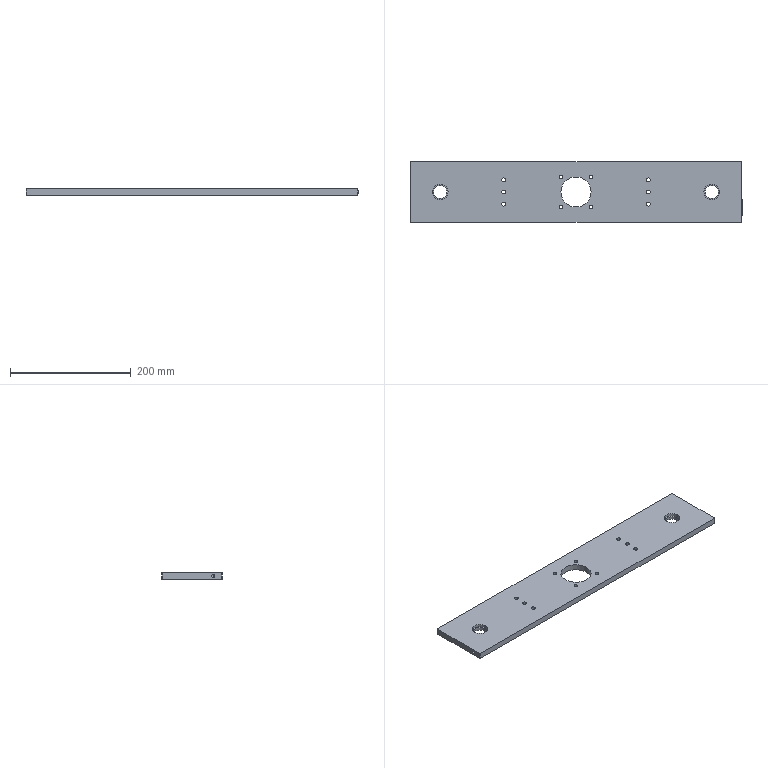Part | SolidWorks | features ICE 5, Extrusion 1, Fillet 1, HoleWzd 1, MirrorPattern 1 | 1 solid | 50 faces | box 550 x 100 x 10 mm | volume 517578 mm3 | cylinder 38 | plane 8 | cone 4 | commonest cylinder face diameters 6.5 x12 5.5 x8 2 x4 5 x4 22 x4 26 x4